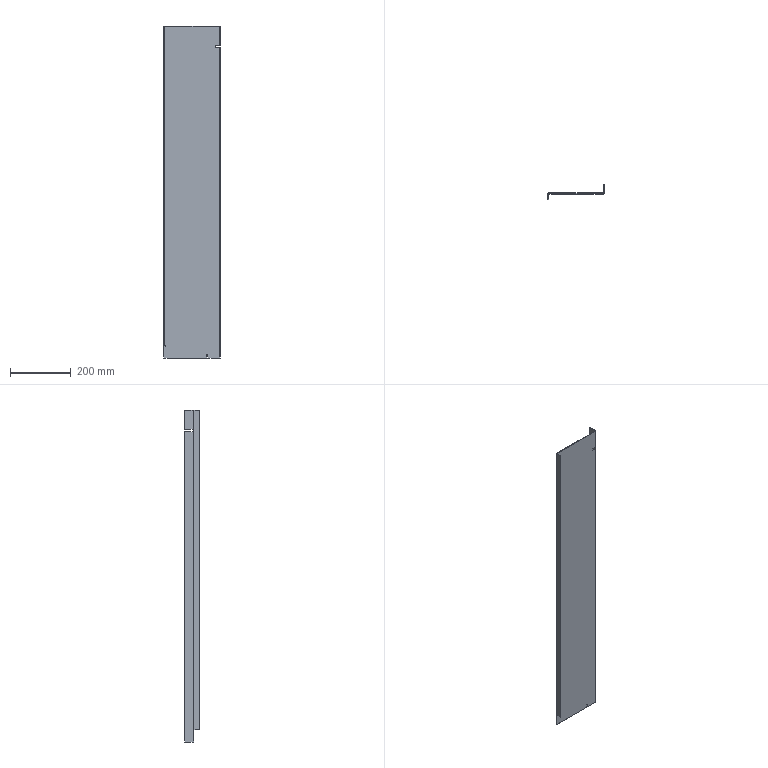Part | STEP file | Right Base Frame | 1 solid | 30 faces | box 185 x 48 x 1095 mm | volume 500987 mm3 | plane 23 | cylinder 7 | commonest cylinder face diameters 1 x4 5 x3
STEP:
#1=CARTESIAN_POINT('',(35.894,0.,57.218));
#2=VERTEX_POINT('',#1);
#3=CARTESIAN_POINT('',(35.894,0.,-966.782));
#4=VERTEX_POINT('',#3);
#5=CARTESIAN_POINT('',(35.894,0.,0.));
#6=DIRECTION('',(0.,0.,-1.));
#7=VECTOR('',#6,1000.);
#8=LINE('',#5,#7);
#9=EDGE_CURVE('',#2,#4,#8,.T.);
#10=ORIENTED_EDGE('',*,*,#9,.T.);
#11=CARTESIAN_POINT('',(-1.606,0.,-966.782));
#12=VERTEX_POINT('',#11);
#13=CARTESIAN_POINT('',(0.,0.,-966.782));
#14=DIRECTION('',(-1.,0.,0.));
#15=VECTOR('',#14,1000.);
#16=LINE('',#13,#15);
#17=EDGE_CURVE('',#4,#12,#16,.T.);
#18=ORIENTED_EDGE('',*,*,#17,.T.);
#19=CARTESIAN_POINT('',(-1.606,0.,-956.782));
#20=VERTEX_POINT('',#19);
#21=CARTESIAN_POINT('',(-1.606,0.,0.));
#22=DIRECTION('',(0.,0.,1.));
#23=VECTOR('',#22,1000.);
#24=LINE('',#21,#23);
#25=EDGE_CURVE('',#12,#20,#24,.T.);
#26=ORIENTED_EDGE('',*,*,#25,.T.);
#27=CARTESIAN_POINT('',(-5.606,0.,-956.782));
#28=VERTEX_POINT('',#27);
#29=CARTESIAN_POINT('',(0.,0.,-956.782));
#30=DIRECTION('',(-1.,0.,0.));
#31=VECTOR('',#30,1000.);
#32=LINE('',#29,#31);
#33=EDGE_CURVE('',#20,#28,#32,.T.);
#34=ORIENTED_EDGE('',*,*,#33,.T.);
#35=CARTESIAN_POINT('',(-5.606,0.,-966.782));
#36=VERTEX_POINT('',#35);
#37=CARTESIAN_POINT('',(-5.606,0.,0.));
#38=DIRECTION('',(0.,0.,-1.));
#39=VECTOR('',#38,1000.);
#40=LINE('',#37,#39);
#41=EDGE_CURVE('',#28,#36,#40,.T.);
#42=ORIENTED_EDGE('',*,*,#41,.T.);
#43=CARTESIAN_POINT('',(-146.606,0.,-966.782));
#44=VERTEX_POINT('',#43);
#45=CARTESIAN_POINT('',(0.,0.,-966.782));
#46=DIRECTION('',(-1.,0.,0.));
#47=VECTOR('',#46,1000.);
#48=LINE('',#45,#47);
#49=EDGE_CURVE('',#36,#44,#48,.T.);
#50=ORIENTED_EDGE('',*,*,#49,.T.);
#51=CARTESIAN_POINT('',(-146.606,0.,-927.782));
#52=VERTEX_POINT('',#51);
#53=CARTESIAN_POINT('',(-146.606,0.,0.));
#54=DIRECTION('',(0.,0.,1.));
#55=VECTOR('',#54,1000.);
#56=LINE('',#53,#55);
#57=EDGE_CURVE('',#44,#52,#56,.T.);
#58=ORIENTED_EDGE('',*,*,#57,.T.);
#59=CARTESIAN_POINT('',(-143.106,0.,-927.782));
#60=VERTEX_POINT('',#59);
#61=CARTESIAN_POINT('',(0.,0.,-927.782));
#62=DIRECTION('',(1.,0.,0.));
#63=VECTOR('',#62,1000.);
#64=LINE('',#61,#63);
#65=EDGE_CURVE('',#52,#60,#64,.T.);
#66=ORIENTED_EDGE('',*,*,#65,.T.);
#67=CARTESIAN_POINT('',(-143.106,0.,-926.782));
#68=VERTEX_POINT('',#67);
#69=CARTESIAN_POINT('',(-143.106,0.,-927.282));
#70=DIRECTION('',(0.,-1.,0.));
#71=DIRECTION('',(0.,0.,1.));
#72=AXIS2_PLACEMENT_3D('',#69,#70,#71);
#73=CIRCLE('',#72,0.5);
#74=EDGE_CURVE('',#60,#68,#73,.T.);
#75=ORIENTED_EDGE('',*,*,#74,.T.);
#76=CARTESIAN_POINT('',(-144.106,0.,-926.782));
#77=VERTEX_POINT('',#76);
#78=CARTESIAN_POINT('',(-143.106,0.,-926.782));
#79=DIRECTION('',(1.,0.,0.));
#80=VECTOR('',#79,1000.);
#81=LINE('',#78,#80);
#82=EDGE_CURVE('',#77,#68,#81,.T.);
#83=ORIENTED_EDGE('',*,*,#82,.F.);
#84=CARTESIAN_POINT('',(-144.106,0.,128.218));
#85=VERTEX_POINT('',#84);
#86=CARTESIAN_POINT('',(-144.106,0.,0.));
#87=DIRECTION('',(0.,0.,1.));
#88=VECTOR('',#87,1000.);
#89=LINE('',#86,#88);
#90=EDGE_CURVE('',#77,#85,#89,.T.);
#91=ORIENTED_EDGE('',*,*,#90,.T.);
#92=CARTESIAN_POINT('',(35.894,0.,128.218));
#93=VERTEX_POINT('',#92);
#94=CARTESIAN_POINT('',(0.,0.,128.218));
#95=DIRECTION('',(1.,0.,0.));
#96=VECTOR('',#95,1000.);
#97=LINE('',#94,#96);
#98=EDGE_CURVE('',#85,#93,#97,.T.);
#99=ORIENTED_EDGE('',*,*,#98,.T.);
#100=CARTESIAN_POINT('',(35.894,0.,64.218));
#101=VERTEX_POINT('',#100);
#102=CARTESIAN_POINT('',(35.894,0.,0.));
#103=DIRECTION('',(0.,0.,-1.));
#104=VECTOR('',#103,1000.);
#105=LINE('',#102,#104);
#106=EDGE_CURVE('',#93,#101,#105,.T.);
#107=ORIENTED_EDGE('',*,*,#106,.T.);
#108=CARTESIAN_POINT('',(22.394,0.,64.218));
#109=VERTEX_POINT('',#108);
#110=CARTESIAN_POINT('',(0.,0.,64.218));
#111=DIRECTION('',(-1.,0.,0.));
#112=VECTOR('',#111,1000.);
#113=LINE('',#110,#112);
#114=EDGE_CURVE('',#101,#109,#113,.T.);
#115=ORIENTED_EDGE('',*,*,#114,.T.);
#116=CARTESIAN_POINT('',(22.394,0.,57.218));
#117=VERTEX_POINT('',#116);
#118=CARTESIAN_POINT('',(22.394,0.,0.));
#119=DIRECTION('',(0.,0.,-1.));
#120=VECTOR('',#119,1000.);
#121=LINE('',#118,#120);
#122=EDGE_CURVE('',#109,#117,#121,.T.);
#123=ORIENTED_EDGE('',*,*,#122,.T.);
#124=CARTESIAN_POINT('',(0.,0.,57.218));
#125=DIRECTION('',(1.,0.,0.));
#126=VECTOR('',#125,1000.);
#127=LINE('',#124,#126);
#128=EDGE_CURVE('',#117,#2,#127,.T.);
#129=ORIENTED_EDGE('',*,*,#128,.T.);
#130=EDGE_LOOP('',(#10,#18,#26,#34,#42,#50,#58,#66,#75,#83,#91,#99,#107,#115,#123,#129));
#131=FACE_OUTER_BOUND('',#130,.T.);
#132=CARTESIAN_POINT('',(0.,0.,0.));
#133=DIRECTION('',(0.,1.,0.));
#134=DIRECTION('',(0.,0.,1.));
#135=AXIS2_PLACEMENT_3D('',#132,#133,#134);
#136=PLANE('',#135);
#137=ADVANCED_FACE('',(#131),#136,.T.);
#138=ORIENTED_EDGE('',*,*,#17,.F.);
#139=CARTESIAN_POINT('',(36.394,0.5,-966.782));
#140=VERTEX_POINT('',#139);
#141=CARTESIAN_POINT('',(35.894,0.5,-966.782));
#142=DIRECTION('',(0.,0.,1.));
#143=DIRECTION('',(-1.,0.,0.));
#144=AXIS2_PLACEMENT_3D('',#141,#142,#143);
#145=CIRCLE('',#144,0.5);
#146=EDGE_CURVE('',#4,#140,#145,.T.);
#147=ORIENTED_EDGE('',*,*,#146,.T.);
#148=CARTESIAN_POINT('',(36.394,28.,-966.782));
#149=VERTEX_POINT('',#148);
#150=CARTESIAN_POINT('',(36.394,0.,-966.782));
#151=DIRECTION('',(0.,-1.,0.));
#152=VECTOR('',#151,1000.);
#153=LINE('',#150,#152);
#154=EDGE_CURVE('',#149,#140,#153,.T.);
#155=ORIENTED_EDGE('',*,*,#154,.F.);
#156=CARTESIAN_POINT('',(38.394,28.,-966.782));
#157=VERTEX_POINT('',#156);
#158=CARTESIAN_POINT('',(38.394,28.,-966.782));
#159=DIRECTION('',(1.,0.,0.));
#160=VECTOR('',#159,1000.);
#161=LINE('',#158,#160);
#162=EDGE_CURVE('',#149,#157,#161,.T.);
#163=ORIENTED_EDGE('',*,*,#162,.T.);
#164=CARTESIAN_POINT('',(38.394,0.5,-966.782));
#165=VERTEX_POINT('',#164);
#166=CARTESIAN_POINT('',(38.394,0.,-966.782));
#167=DIRECTION('',(0.,-1.,0.));
#168=VECTOR('',#167,1000.);
#169=LINE('',#166,#168);
#170=EDGE_CURVE('',#157,#165,#169,.T.);
#171=ORIENTED_EDGE('',*,*,#170,.T.);
#172=CARTESIAN_POINT('',(35.894,-2.,-966.782));
#173=VERTEX_POINT('',#172);
#174=CARTESIAN_POINT('',(35.894,0.5,-966.782));
#175=DIRECTION('',(0.,0.,1.));
#176=DIRECTION('',(-1.,0.,0.));
#177=AXIS2_PLACEMENT_3D('',#174,#175,#176);
#178=CIRCLE('',#177,2.5);
#179=EDGE_CURVE('',#173,#165,#178,.T.);
#180=ORIENTED_EDGE('',*,*,#179,.F.);
#181=CARTESIAN_POINT('',(-1.606,-2.,-966.782));
#182=VERTEX_POINT('',#181);
#183=CARTESIAN_POINT('',(-146.606,-2.,-966.782));
#184=DIRECTION('',(-1.,0.,0.));
#185=VECTOR('',#184,1000.);
#186=LINE('',#183,#185);
#187=EDGE_CURVE('',#173,#182,#186,.T.);
#188=ORIENTED_EDGE('',*,*,#187,.T.);
#189=CARTESIAN_POINT('',(-1.606,-2.,-966.782));
#190=DIRECTION('',(0.,1.,0.));
#191=VECTOR('',#190,1000.);
#192=LINE('',#189,#191);
#193=EDGE_CURVE('',#182,#12,#192,.T.);
#194=ORIENTED_EDGE('',*,*,#193,.T.);
#195=EDGE_LOOP('',(#138,#147,#155,#163,#171,#180,#188,#194));
#196=FACE_OUTER_BOUND('',#195,.T.);
#197=CARTESIAN_POINT('',(-146.606,-2.,-966.782));
#198=DIRECTION('',(0.,0.,-1.));
#199=DIRECTION('',(-1.,0.,0.));
#200=AXIS2_PLACEMENT_3D('',#197,#198,#199);
#201=PLANE('',#200);
#202=ADVANCED_FACE('',(#196),#201,.T.);
#203=CARTESIAN_POINT('',(36.394,0.5,57.218));
#204=VERTEX_POINT('',#203);
#205=CARTESIAN_POINT('',(35.894,0.5,57.218));
#206=DIRECTION('',(0.,0.,-1.));
#207=DIRECTION('',(-1.,0.,0.));
#208=AXIS2_PLACEMENT_3D('',#205,#206,#207);
#209=CIRCLE('',#208,0.5);
#210=EDGE_CURVE('',#204,#2,#209,.T.);
#211=ORIENTED_EDGE('',*,*,#210,.F.);
#212=CARTESIAN_POINT('',(36.394,0.5,-966.782));
#213=DIRECTION('',(0.,0.,1.));
#214=VECTOR('',#213,1000.);
#215=LINE('',#212,#214);
#216=EDGE_CURVE('',#140,#204,#215,.T.);
#217=ORIENTED_EDGE('',*,*,#216,.F.);
#218=ORIENTED_EDGE('',*,*,#146,.F.);
#219=ORIENTED_EDGE('',*,*,#9,.F.);
#220=EDGE_LOOP('',(#211,#217,#218,#219));
#221=FACE_OUTER_BOUND('',#220,.T.);
#222=CARTESIAN_POINT('',(35.894,0.5,-966.782));
#223=DIRECTION('',(0.,0.,-1.));
#224=DIRECTION('',(-1.,0.,0.));
#225=AXIS2_PLACEMENT_3D('',#222,#223,#224);
#226=CYLINDRICAL_SURFACE('',#225,0.5);
#227=ADVANCED_FACE('',(#221),#226,.F.);
#228=CARTESIAN_POINT('',(38.394,28.,57.218));
#229=VERTEX_POINT('',#228);
#230=CARTESIAN_POINT('',(38.394,0.5,57.218));
#231=VERTEX_POINT('',#230);
#232=CARTESIAN_POINT('',(38.394,-20.,57.218));
#233=DIRECTION('',(0.,-1.,0.));
#234=VECTOR('',#233,1000.);
#235=LINE('',#232,#234);
#236=EDGE_CURVE('',#229,#231,#235,.T.);
#237=ORIENTED_EDGE('',*,*,#236,.F.);
#238=CARTESIAN_POINT('',(36.394,28.,57.218));
#239=VERTEX_POINT('',#238);
#240=CARTESIAN_POINT('',(38.394,28.,57.218));
#241=DIRECTION('',(1.,0.,0.));
#242=VECTOR('',#241,1000.);
#243=LINE('',#240,#242);
#244=EDGE_CURVE('',#239,#229,#243,.T.);
#245=ORIENTED_EDGE('',*,*,#244,.F.);
#246=CARTESIAN_POINT('',(36.394,-20.,57.218));
#247=DIRECTION('',(0.,1.,0.));
#248=VECTOR('',#247,1000.);
#249=LINE('',#246,#248);
#250=EDGE_CURVE('',#204,#239,#249,.T.);
#251=ORIENTED_EDGE('',*,*,#250,.F.);
#252=ORIENTED_EDGE('',*,*,#210,.T.);
#253=ORIENTED_EDGE('',*,*,#128,.F.);
#254=CARTESIAN_POINT('',(22.394,-2.,57.218));
#255=VERTEX_POINT('',#254);
#256=CARTESIAN_POINT('',(22.394,-20.,57.218));
#257=DIRECTION('',(0.,1.,0.));
#258=VECTOR('',#257,1000.);
#259=LINE('',#256,#258);
#260=EDGE_CURVE('',#255,#117,#259,.T.);
#261=ORIENTED_EDGE('',*,*,#260,.F.);
#262=CARTESIAN_POINT('',(35.894,-2.,57.218));
#263=VERTEX_POINT('',#262);
#264=CARTESIAN_POINT('',(38.394,-2.,57.218));
#265=DIRECTION('',(-1.,0.,0.));
#266=VECTOR('',#265,1000.);
#267=LINE('',#264,#266);
#268=EDGE_CURVE('',#263,#255,#267,.T.);
#269=ORIENTED_EDGE('',*,*,#268,.F.);
#270=CARTESIAN_POINT('',(35.894,0.5,57.218));
#271=DIRECTION('',(0.,0.,-1.));
#272=DIRECTION('',(-1.,0.,0.));
#273=AXIS2_PLACEMENT_3D('',#270,#271,#272);
#274=CIRCLE('',#273,2.5);
#275=EDGE_CURVE('',#231,#263,#274,.T.);
#276=ORIENTED_EDGE('',*,*,#275,.F.);
#277=EDGE_LOOP('',(#237,#245,#251,#252,#253,#261,#269,#276));
#278=FACE_OUTER_BOUND('',#277,.T.);
#279=CARTESIAN_POINT('',(38.394,-20.,57.218));
#280=DIRECTION('',(0.,0.,-1.));
#281=DIRECTION('',(-1.,0.,0.));
#282=AXIS2_PLACEMENT_3D('',#279,#280,#281);
#283=PLANE('',#282);
#284=ADVANCED_FACE('',(#278),#283,.F.);
#285=ORIENTED_EDGE('',*,*,#122,.F.);
#286=CARTESIAN_POINT('',(22.394,-2.,64.218));
#287=VERTEX_POINT('',#286);
#288=CARTESIAN_POINT('',(22.394,-20.,64.218));
#289=DIRECTION('',(0.,1.,0.));
#290=VECTOR('',#289,1000.);
#291=LINE('',#288,#290);
#292=EDGE_CURVE('',#287,#109,#291,.T.);
#293=ORIENTED_EDGE('',*,*,#292,.F.);
#294=CARTESIAN_POINT('',(22.394,-2.,57.218));
#295=DIRECTION('',(0.,0.,1.));
#296=VECTOR('',#295,1000.);
#297=LINE('',#294,#296);
#298=EDGE_CURVE('',#255,#287,#297,.T.);
#299=ORIENTED_EDGE('',*,*,#298,.F.);
#300=ORIENTED_EDGE('',*,*,#260,.T.);
#301=EDGE_LOOP('',(#285,#293,#299,#300));
#302=FACE_OUTER_BOUND('',#301,.T.);
#303=CARTESIAN_POINT('',(22.394,-20.,57.218));
#304=DIRECTION('',(-1.,0.,0.));
#305=DIRECTION('',(0.,-1.,0.));
#306=AXIS2_PLACEMENT_3D('',#303,#304,#305);
#307=PLANE('',#306);
#308=ADVANCED_FACE('',(#302),#307,.F.);
#309=ORIENTED_EDGE('',*,*,#114,.F.);
#310=CARTESIAN_POINT('',(36.394,0.5,64.218));
#311=VERTEX_POINT('',#310);
#312=CARTESIAN_POINT('',(35.894,0.5,64.218));
#313=DIRECTION('',(0.,0.,-1.));
#314=DIRECTION('',(-1.,0.,0.));
#315=AXIS2_PLACEMENT_3D('',#312,#313,#314);
#316=CIRCLE('',#315,0.5);
#317=EDGE_CURVE('',#311,#101,#316,.T.);
#318=ORIENTED_EDGE('',*,*,#317,.F.);
#319=CARTESIAN_POINT('',(36.394,28.,64.218));
#320=VERTEX_POINT('',#319);
#321=CARTESIAN_POINT('',(36.394,-20.,64.218));
#322=DIRECTION('',(0.,-1.,0.));
#323=VECTOR('',#322,1000.);
#324=LINE('',#321,#323);
#325=EDGE_CURVE('',#320,#311,#324,.T.);
#326=ORIENTED_EDGE('',*,*,#325,.F.);
#327=CARTESIAN_POINT('',(38.394,28.,64.218));
#328=VERTEX_POINT('',#327);
#329=CARTESIAN_POINT('',(38.394,28.,64.218));
#330=DIRECTION('',(-1.,0.,0.));
#331=VECTOR('',#330,1000.);
#332=LINE('',#329,#331);
#333=EDGE_CURVE('',#328,#320,#332,.T.);
#334=ORIENTED_EDGE('',*,*,#333,.F.);
#335=CARTESIAN_POINT('',(38.394,0.5,64.218));
#336=VERTEX_POINT('',#335);
#337=CARTESIAN_POINT('',(38.394,-20.,64.218));
#338=DIRECTION('',(0.,1.,0.));
#339=VECTOR('',#338,1000.);
#340=LINE('',#337,#339);
#341=EDGE_CURVE('',#336,#328,#340,.T.);
#342=ORIENTED_EDGE('',*,*,#341,.F.);
#343=CARTESIAN_POINT('',(35.894,-2.,64.218));
#344=VERTEX_POINT('',#343);
#345=CARTESIAN_POINT('',(35.894,0.5,64.218));
#346=DIRECTION('',(0.,0.,1.));
#347=DIRECTION('',(-1.,0.,0.));
#348=AXIS2_PLACEMENT_3D('',#345,#346,#347);
#349=CIRCLE('',#348,2.5);
#350=EDGE_CURVE('',#344,#336,#349,.T.);
#351=ORIENTED_EDGE('',*,*,#350,.F.);
#352=CARTESIAN_POINT('',(38.394,-2.,64.218));
#353=DIRECTION('',(1.,0.,0.));
#354=VECTOR('',#353,1000.);
#355=LINE('',#352,#354);
#356=EDGE_CURVE('',#287,#344,#355,.T.);
#357=ORIENTED_EDGE('',*,*,#356,.F.);
#358=ORIENTED_EDGE('',*,*,#292,.T.);
#359=EDGE_LOOP('',(#309,#318,#326,#334,#342,#351,#357,#358));
#360=FACE_OUTER_BOUND('',#359,.T.);
#361=CARTESIAN_POINT('',(38.394,-20.,64.218));
#362=DIRECTION('',(0.,0.,1.));
#363=DIRECTION('',(0.,-1.,0.));
#364=AXIS2_PLACEMENT_3D('',#361,#362,#363);
#365=PLANE('',#364);
#366=ADVANCED_FACE('',(#360),#365,.F.);
#367=ORIENTED_EDGE('',*,*,#317,.T.);
#368=ORIENTED_EDGE('',*,*,#106,.F.);
#369=CARTESIAN_POINT('',(36.394,0.5,128.218));
#370=VERTEX_POINT('',#369);
#371=CARTESIAN_POINT('',(35.894,0.5,128.218));
#372=DIRECTION('',(0.,0.,-1.));
#373=DIRECTION('',(-1.,0.,0.));
#374=AXIS2_PLACEMENT_3D('',#371,#372,#373);
#375=CIRCLE('',#374,0.5);
#376=EDGE_CURVE('',#370,#93,#375,.T.);
#377=ORIENTED_EDGE('',*,*,#376,.F.);
#378=CARTESIAN_POINT('',(36.394,0.5,-966.782));
#379=DIRECTION('',(0.,0.,1.));
#380=VECTOR('',#379,1000.);
#381=LINE('',#378,#380);
#382=EDGE_CURVE('',#311,#370,#381,.T.);
#383=ORIENTED_EDGE('',*,*,#382,.F.);
#384=EDGE_LOOP('',(#367,#368,#377,#383));
#385=FACE_OUTER_BOUND('',#384,.T.);
#386=CARTESIAN_POINT('',(35.894,0.5,-966.782));
#387=DIRECTION('',(0.,0.,-1.));
#388=DIRECTION('',(-1.,0.,0.));
#389=AXIS2_PLACEMENT_3D('',#386,#387,#388);
#390=CYLINDRICAL_SURFACE('',#389,0.5);
#391=ADVANCED_FACE('',(#385),#390,.F.);
#392=ORIENTED_EDGE('',*,*,#98,.F.);
#393=CARTESIAN_POINT('',(-146.606,-2.5,128.218));
#394=VERTEX_POINT('',#393);
#395=CARTESIAN_POINT('',(-144.106,-2.5,128.218));
#396=DIRECTION('',(0.,0.,-1.));
#397=DIRECTION('',(0.,1.,0.));
#398=AXIS2_PLACEMENT_3D('',#395,#396,#397);
#399=CIRCLE('',#398,2.5);
#400=EDGE_CURVE('',#394,#85,#399,.T.);
#401=ORIENTED_EDGE('',*,*,#400,.F.);
#402=CARTESIAN_POINT('',(-146.606,-20.,128.218));
#403=VERTEX_POINT('',#402);
#404=CARTESIAN_POINT('',(-146.606,0.,128.218));
#405=DIRECTION('',(0.,1.,0.));
#406=VECTOR('',#405,1000.);
#407=LINE('',#404,#406);
#408=EDGE_CURVE('',#403,#394,#407,.T.);
#409=ORIENTED_EDGE('',*,*,#408,.F.);
#410=CARTESIAN_POINT('',(-144.606,-20.,128.218));
#411=VERTEX_POINT('',#410);
#412=CARTESIAN_POINT('',(-146.606,-20.,128.218));
#413=DIRECTION('',(1.,0.,0.));
#414=VECTOR('',#413,1000.);
#415=LINE('',#412,#414);
#416=EDGE_CURVE('',#403,#411,#415,.T.);
#417=ORIENTED_EDGE('',*,*,#416,.T.);
#418=CARTESIAN_POINT('',(-144.606,-2.5,128.218));
#419=VERTEX_POINT('',#418);
#420=CARTESIAN_POINT('',(-144.606,-20.,128.218));
#421=DIRECTION('',(0.,1.,0.));
#422=VECTOR('',#421,1000.);
#423=LINE('',#420,#422);
#424=EDGE_CURVE('',#411,#419,#423,.T.);
#425=ORIENTED_EDGE('',*,*,#424,.T.);
#426=CARTESIAN_POINT('',(-144.106,-2.,128.218));
#427=VERTEX_POINT('',#426);
#428=CARTESIAN_POINT('',(-144.106,-2.5,128.218));
#429=DIRECTION('',(0.,0.,-1.));
#430=DIRECTION('',(0.,1.,0.));
#431=AXIS2_PLACEMENT_3D('',#428,#429,#430);
#432=CIRCLE('',#431,0.5);
#433=EDGE_CURVE('',#419,#427,#432,.T.);
#434=ORIENTED_EDGE('',*,*,#433,.T.);
#435=CARTESIAN_POINT('',(35.894,-2.,128.218));
#436=VERTEX_POINT('',#435);
#437=CARTESIAN_POINT('',(-146.606,-2.,128.218));
#438=DIRECTION('',(1.,0.,0.));
#439=VECTOR('',#438,1000.);
#440=LINE('',#437,#439);
#441=EDGE_CURVE('',#427,#436,#440,.T.);
#442=ORIENTED_EDGE('',*,*,#441,.T.);
#443=CARTESIAN_POINT('',(38.394,0.5,128.218));
#444=VERTEX_POINT('',#443);
#445=CARTESIAN_POINT('',(35.894,0.5,128.218));
#446=DIRECTION('',(0.,0.,-1.));
#447=DIRECTION('',(-1.,0.,0.));
#448=AXIS2_PLACEMENT_3D('',#445,#446,#447);
#449=CIRCLE('',#448,2.5);
#450=EDGE_CURVE('',#444,#436,#449,.T.);
#451=ORIENTED_EDGE('',*,*,#450,.F.);
#452=CARTESIAN_POINT('',(38.394,28.,128.218));
#453=VERTEX_POINT('',#452);
#454=CARTESIAN_POINT('',(38.394,0.,128.218));
#455=DIRECTION('',(0.,1.,0.));
#456=VECTOR('',#455,1000.);
#457=LINE('',#454,#456);
#458=EDGE_CURVE('',#444,#453,#457,.T.);
#459=ORIENTED_EDGE('',*,*,#458,.T.);
#460=CARTESIAN_POINT('',(36.394,28.,128.218));
#461=VERTEX_POINT('',#460);
#462=CARTESIAN_POINT('',(38.394,28.,128.218));
#463=DIRECTION('',(-1.,0.,0.));
#464=VECTOR('',#463,1000.);
#465=LINE('',#462,#464);
#466=EDGE_CURVE('',#453,#461,#465,.T.);
#467=ORIENTED_EDGE('',*,*,#466,.T.);
#468=CARTESIAN_POINT('',(36.394,0.,128.218));
#469=DIRECTION('',(0.,1.,0.));
#470=VECTOR('',#469,1000.);
#471=LINE('',#468,#470);
#472=EDGE_CURVE('',#370,#461,#471,.T.);
#473=ORIENTED_EDGE('',*,*,#472,.F.);
#474=ORIENTED_EDGE('',*,*,#376,.T.);
#475=EDGE_LOOP('',(#392,#401,#409,#417,#425,#434,#442,#451,#459,#467,#473,#474));
#476=FACE_OUTER_BOUND('',#475,.T.);
#477=CARTESIAN_POINT('',(-146.606,-2.,128.218));
#478=DIRECTION('',(0.,0.,1.));
#479=DIRECTION('',(1.,0.,0.));
#480=AXIS2_PLACEMENT_3D('',#477,#478,#479);
#481=PLANE('',#480);
#482=ADVANCED_FACE('',(#476),#481,.T.);
#483=CARTESIAN_POINT('',(-146.606,-2.5,-926.782));
#484=VERTEX_POINT('',#483);
#485=CARTESIAN_POINT('',(-146.606,-2.5,-926.782));
#486=DIRECTION('',(0.,0.,1.));
#487=VECTOR('',#486,1000.);
#488=LINE('',#485,#487);
#489=EDGE_CURVE('',#484,#394,#488,.T.);
#490=ORIENTED_EDGE('',*,*,#489,.T.);
#491=ORIENTED_EDGE('',*,*,#400,.T.);
#492=ORIENTED_EDGE('',*,*,#90,.F.);
#493=CARTESIAN_POINT('',(-144.106,-2.5,-926.782));
#494=DIRECTION('',(0.,0.,1.));
#495=DIRECTION('',(0.,1.,0.));
#496=AXIS2_PLACEMENT_3D('',#493,#494,#495);
#497=CIRCLE('',#496,2.5);
#498=EDGE_CURVE('',#77,#484,#497,.T.);
#499=ORIENTED_EDGE('',*,*,#498,.T.);
#500=EDGE_LOOP('',(#490,#491,#492,#499));
#501=FACE_OUTER_BOUND('',#500,.T.);
#502=CARTESIAN_POINT('',(-144.106,-2.5,-926.782));
#503=DIRECTION('',(0.,0.,-1.));
#504=DIRECTION('',(0.,1.,0.));
#505=AXIS2_PLACEMENT_3D('',#502,#503,#504);
#506=CYLINDRICAL_SURFACE('',#505,2.5);
#507=ADVANCED_FACE('',(#501),#506,.T.);
#508=CARTESIAN_POINT('',(-146.606,-2.,-927.782));
#509=VERTEX_POINT('',#508);
#510=CARTESIAN_POINT('',(-143.106,-2.,-927.782));
#511=VERTEX_POINT('',#510);
#512=CARTESIAN_POINT('',(-146.606,-2.,-927.782));
#513=DIRECTION('',(1.,0.,0.));
#514=VECTOR('',#513,1000.);
#515=LINE('',#512,#514);
#516=EDGE_CURVE('',#509,#511,#515,.T.);
#517=ORIENTED_EDGE('',*,*,#516,.T.);
#518=CARTESIAN_POINT('',(-143.106,-2.,-927.782));
#519=DIRECTION('',(0.,1.,0.));
#520=VECTOR('',#519,1000.);
#521=LINE('',#518,#520);
#522=EDGE_CURVE('',#511,#60,#521,.T.);
#523=ORIENTED_EDGE('',*,*,#522,.T.);
#524=ORIENTED_EDGE('',*,*,#65,.F.);
#525=CARTESIAN_POINT('',(-146.606,-2.,-927.782));
#526=DIRECTION('',(0.,-1.,0.));
#527=VECTOR('',#526,1000.);
#528=LINE('',#525,#527);
#529=EDGE_CURVE('',#52,#509,#528,.T.);
#530=ORIENTED_EDGE('',*,*,#529,.T.);
#531=EDGE_LOOP('',(#517,#523,#524,#530));
#532=FACE_OUTER_BOUND('',#531,.T.);
#533=CARTESIAN_POINT('',(-146.606,-2.,-927.782));
#534=DIRECTION('',(0.,0.,1.));
#535=DIRECTION('',(0.,-1.,0.));
#536=AXIS2_PLACEMENT_3D('',#533,#534,#535);
#537=PLANE('',#536);
#538=ADVANCED_FACE('',(#532),#537,.T.);
#539=ORIENTED_EDGE('',*,*,#57,.F.);
#540=CARTESIAN_POINT('',(-146.606,-2.,-966.782));
#541=VERTEX_POINT('',#540);
#542=CARTESIAN_POINT('',(-146.606,-2.,-966.782));
#543=DIRECTION('',(0.,-1.,0.));
#544=VECTOR('',#543,1000.);
#545=LINE('',#542,#544);
#546=EDGE_CURVE('',#44,#541,#545,.T.);
#547=ORIENTED_EDGE('',*,*,#546,.T.);
#548=CARTESIAN_POINT('',(-146.606,-2.,-966.782));
#549=DIRECTION('',(0.,0.,1.));
#550=VECTOR('',#549,1000.);
#551=LINE('',#548,#550);
#552=EDGE_CURVE('',#541,#509,#551,.T.);
#553=ORIENTED_EDGE('',*,*,#552,.T.);
#554=ORIENTED_EDGE('',*,*,#529,.F.);
#555=EDGE_LOOP('',(#539,#547,#553,#554));
#556=FACE_OUTER_BOUND('',#555,.T.);
#557=CARTESIAN_POINT('',(-146.606,-2.,-966.782));
#558=DIRECTION('',(-1.,0.,0.));
#559=DIRECTION('',(0.,0.,1.));
#560=AXIS2_PLACEMENT_3D('',#557,#558,#559);
#561=PLANE('',#560);
#562=ADVANCED_FACE('',(#556),#561,.T.);
#563=ORIENTED_EDGE('',*,*,#546,.F.);
#564=ORIENTED_EDGE('',*,*,#49,.F.);
#565=CARTESIAN_POINT('',(-5.606,-2.,-966.782));
#566=VERTEX_POINT('',#565);
#567=CARTESIAN_POINT('',(-5.606,-2.,-966.782));
#568=DIRECTION('',(0.,-1.,0.));
#569=VECTOR('',#568,1000.);
#570=LINE('',#567,#569);
#571=EDGE_CURVE('',#36,#566,#570,.T.);
#572=ORIENTED_EDGE('',*,*,#571,.T.);
#573=CARTESIAN_POINT('',(-146.606,-2.,-966.782));
#574=DIRECTION('',(-1.,0.,0.));
#575=VECTOR('',#574,1000.);
#576=LINE('',#573,#575);
#577=EDGE_CURVE('',#566,#541,#576,.T.);
#578=ORIENTED_EDGE('',*,*,#577,.T.);
#579=EDGE_LOOP('',(#563,#564,#572,#578));
#580=FACE_OUTER_BOUND('',#579,.T.);
#581=CARTESIAN_POINT('',(-146.606,-2.,-966.782));
#582=DIRECTION('',(0.,0.,-1.));
#583=DIRECTION('',(-1.,0.,0.));
#584=AXIS2_PLACEMENT_3D('',#581,#582,#583);
#585=PLANE('',#584);
#586=ADVANCED_FACE('',(#580),#585,.T.);
#587=ORIENTED_EDGE('',*,*,#41,.F.);
#588=CARTESIAN_POINT('',(-5.606,-2.,-956.782));
#589=VERTEX_POINT('',#588);
#590=CARTESIAN_POINT('',(-5.606,-10.,-956.782));
#591=DIRECTION('',(0.,1.,0.));
#592=VECTOR('',#591,1000.);
#593=LINE('',#590,#592);
#594=EDGE_CURVE('',#589,#28,#593,.T.);
#595=ORIENTED_EDGE('',*,*,#594,.F.);
#596=CARTESIAN_POINT('',(-5.606,-2.,-966.782));
#597=DIRECTION('',(0.,0.,1.));
#598=VECTOR('',#597,1000.);
#599=LINE('',#596,#598);
#600=EDGE_CURVE('',#566,#589,#599,.T.);
#601=ORIENTED_EDGE('',*,*,#600,.F.);
#602=ORIENTED_EDGE('',*,*,#571,.F.);
#603=EDGE_LOOP('',(#587,#595,#601,#602));
#604=FACE_OUTER_BOUND('',#603,.T.);
#605=CARTESIAN_POINT('',(-5.606,-10.,-966.782));
#606=DIRECTION('',(-1.,0.,0.));
#607=DIRECTION('',(0.,0.,1.));
#608=AXIS2_PLACEMENT_3D('',#605,#606,#607);
#609=PLANE('',#608);
#610=ADVANCED_FACE('',(#604),#609,.F.);
#611=ORIENTED_EDGE('',*,*,#33,.F.);
#612=CARTESIAN_POINT('',(-1.606,-2.,-956.782));
#613=VERTEX_POINT('',#612);
#614=CARTESIAN_POINT('',(-1.606,-10.,-956.782));
#615=DIRECTION('',(0.,1.,0.));
#616=VECTOR('',#615,1000.);
#617=LINE('',#614,#616);
#618=EDGE_CURVE('',#613,#20,#617,.T.);
#619=ORIENTED_EDGE('',*,*,#618,.F.);
#620=CARTESIAN_POINT('',(-1.606,-2.,-956.782));
#621=DIRECTION('',(1.,0.,0.));
#622=VECTOR('',#621,1000.);
#623=LINE('',#620,#622);
#624=EDGE_CURVE('',#589,#613,#623,.T.);
#625=ORIENTED_EDGE('',*,*,#624,.F.);
#626=ORIENTED_EDGE('',*,*,#594,.T.);
#627=EDGE_LOOP('',(#611,#619,#625,#626));
#628=FACE_OUTER_BOUND('',#627,.T.);
#629=CARTESIAN_POINT('',(-1.606,-10.,-956.782));
#630=DIRECTION('',(0.,0.,1.));
#631=DIRECTION('',(1.,0.,0.));
#632=AXIS2_PLACEMENT_3D('',#629,#630,#631);
#633=PLANE('',#632);
#634=ADVANCED_FACE('',(#628),#633,.F.);
#635=ORIENTED_EDGE('',*,*,#25,.F.);
#636=ORIENTED_EDGE('',*,*,#193,.F.);
#637=CARTESIAN_POINT('',(-1.606,-2.,-966.782));
#638=DIRECTION('',(0.,0.,-1.));
#639=VECTOR('',#638,1000.);
#640=LINE('',#637,#639);
#641=EDGE_CURVE('',#613,#182,#640,.T.);
#642=ORIENTED_EDGE('',*,*,#641,.F.);
#643=ORIENTED_EDGE('',*,*,#618,.T.);
#644=EDGE_LOOP('',(#635,#636,#642,#643));
#645=FACE_OUTER_BOUND('',#644,.T.);
#646=CARTESIAN_POINT('',(-1.606,-10.,-966.782));
#647=DIRECTION('',(1.,0.,0.));
#648=DIRECTION('',(0.,0.,-1.));
#649=AXIS2_PLACEMENT_3D('',#646,#647,#648);
#650=PLANE('',#649);
#651=ADVANCED_FACE('',(#645),#650,.F.);
#652=ORIENTED_EDGE('',*,*,#641,.T.);
#653=ORIENTED_EDGE('',*,*,#187,.F.);
#654=CARTESIAN_POINT('',(35.894,-2.,0.));
#655=DIRECTION('',(0.,0.,-1.));
#656=VECTOR('',#655,1000.);
#657=LINE('',#654,#656);
#658=EDGE_CURVE('',#263,#173,#657,.T.);
#659=ORIENTED_EDGE('',*,*,#658,.F.);
#660=ORIENTED_EDGE('',*,*,#268,.T.);
#661=ORIENTED_EDGE('',*,*,#298,.T.);
#662=ORIENTED_EDGE('',*,*,#356,.T.);
#663=CARTESIAN_POINT('',(35.894,-2.,0.));
#664=DIRECTION('',(0.,0.,-1.));
#665=VECTOR('',#664,1000.);
#666=LINE('',#663,#665);
#667=EDGE_CURVE('',#436,#344,#666,.T.);
#668=ORIENTED_EDGE('',*,*,#667,.F.);
#669=ORIENTED_EDGE('',*,*,#441,.F.);
#670=CARTESIAN_POINT('',(-144.106,-2.,-926.782));
#671=VERTEX_POINT('',#670);
#672=CARTESIAN_POINT('',(-144.106,-2.,0.));
#673=DIRECTION('',(0.,0.,1.));
#674=VECTOR('',#673,1000.);
#675=LINE('',#672,#674);
#676=EDGE_CURVE('',#671,#427,#675,.T.);
#677=ORIENTED_EDGE('',*,*,#676,.F.);
#678=CARTESIAN_POINT('',(-143.106,-2.,-926.782));
#679=VERTEX_POINT('',#678);
#680=CARTESIAN_POINT('',(-143.106,-2.,-926.782));
#681=DIRECTION('',(-1.,0.,0.));
#682=VECTOR('',#681,1000.);
#683=LINE('',#680,#682);
#684=EDGE_CURVE('',#679,#671,#683,.T.);
#685=ORIENTED_EDGE('',*,*,#684,.F.);
#686=CARTESIAN_POINT('',(-143.106,-2.,-927.282));
#687=DIRECTION('',(0.,-1.,0.));
#688=DIRECTION('',(0.,0.,1.));
#689=AXIS2_PLACEMENT_3D('',#686,#687,#688);
#690=CIRCLE('',#689,0.5);
#691=EDGE_CURVE('',#511,#679,#690,.T.);
#692=ORIENTED_EDGE('',*,*,#691,.F.);
#693=ORIENTED_EDGE('',*,*,#516,.F.);
#694=ORIENTED_EDGE('',*,*,#552,.F.);
#695=ORIENTED_EDGE('',*,*,#577,.F.);
#696=ORIENTED_EDGE('',*,*,#600,.T.);
#697=ORIENTED_EDGE('',*,*,#624,.T.);
#698=EDGE_LOOP('',(#652,#653,#659,#660,#661,#662,#668,#669,#677,#685,#692,#693,#694,#695,#696,#697));
#699=FACE_OUTER_BOUND('',#698,.T.);
#700=CARTESIAN_POINT('',(0.,-2.,0.));
#701=DIRECTION('',(0.,1.,0.));
#702=DIRECTION('',(0.,0.,1.));
#703=AXIS2_PLACEMENT_3D('',#700,#701,#702);
#704=PLANE('',#703);
#705=ADVANCED_FACE('',(#699),#704,.F.);
#706=ORIENTED_EDGE('',*,*,#154,.T.);
#707=ORIENTED_EDGE('',*,*,#216,.T.);
#708=ORIENTED_EDGE('',*,*,#250,.T.);
#709=CARTESIAN_POINT('',(36.394,28.,0.));
#710=DIRECTION('',(0.,0.,-1.));
#711=VECTOR('',#710,1000.);
#712=LINE('',#709,#711);
#713=EDGE_CURVE('',#239,#149,#712,.T.);
#714=ORIENTED_EDGE('',*,*,#713,.T.);
#715=EDGE_LOOP('',(#706,#707,#708,#714));
#716=FACE_OUTER_BOUND('',#715,.T.);
#717=CARTESIAN_POINT('',(36.394,0.,0.));
#718=DIRECTION('',(-1.,0.,0.));
#719=DIRECTION('',(0.,-1.,0.));
#720=AXIS2_PLACEMENT_3D('',#717,#718,#719);
#721=PLANE('',#720);
#722=ADVANCED_FACE('',(#716),#721,.T.);
#723=ORIENTED_EDGE('',*,*,#179,.T.);
#724=CARTESIAN_POINT('',(38.394,0.5,-966.782));
#725=DIRECTION('',(0.,0.,1.));
#726=VECTOR('',#725,1000.);
#727=LINE('',#724,#726);
#728=EDGE_CURVE('',#165,#231,#727,.T.);
#729=ORIENTED_EDGE('',*,*,#728,.T.);
#730=ORIENTED_EDGE('',*,*,#275,.T.);
#731=ORIENTED_EDGE('',*,*,#658,.T.);
#732=EDGE_LOOP('',(#723,#729,#730,#731));
#733=FACE_OUTER_BOUND('',#732,.T.);
#734=CARTESIAN_POINT('',(35.894,0.5,-966.782));
#735=DIRECTION('',(0.,0.,-1.));
#736=DIRECTION('',(-1.,0.,0.));
#737=AXIS2_PLACEMENT_3D('',#734,#735,#736);
#738=CYLINDRICAL_SURFACE('',#737,2.5);
#739=ADVANCED_FACE('',(#733),#738,.T.);
#740=ORIENTED_EDGE('',*,*,#236,.T.);
#741=ORIENTED_EDGE('',*,*,#728,.F.);
#742=ORIENTED_EDGE('',*,*,#170,.F.);
#743=CARTESIAN_POINT('',(38.394,28.,0.));
#744=DIRECTION('',(0.,0.,-1.));
#745=VECTOR('',#744,1000.);
#746=LINE('',#743,#745);
#747=EDGE_CURVE('',#229,#157,#746,.T.);
#748=ORIENTED_EDGE('',*,*,#747,.F.);
#749=EDGE_LOOP('',(#740,#741,#742,#748));
#750=FACE_OUTER_BOUND('',#749,.T.);
#751=CARTESIAN_POINT('',(38.394,0.,0.));
#752=DIRECTION('',(-1.,0.,0.));
#753=DIRECTION('',(0.,-1.,0.));
#754=AXIS2_PLACEMENT_3D('',#751,#752,#753);
#755=PLANE('',#754);
#756=ADVANCED_FACE('',(#750),#755,.F.);
#757=ORIENTED_EDGE('',*,*,#244,.T.);
#758=ORIENTED_EDGE('',*,*,#747,.T.);
#759=ORIENTED_EDGE('',*,*,#162,.F.);
#760=ORIENTED_EDGE('',*,*,#713,.F.);
#761=EDGE_LOOP('',(#757,#758,#759,#760));
#762=FACE_OUTER_BOUND('',#761,.T.);
#763=CARTESIAN_POINT('',(38.394,28.,128.218));
#764=DIRECTION('',(0.,-1.,0.));
#765=DIRECTION('',(1.,0.,0.));
#766=AXIS2_PLACEMENT_3D('',#763,#764,#765);
#767=PLANE('',#766);
#768=ADVANCED_FACE('',(#762),#767,.F.);
#769=ORIENTED_EDGE('',*,*,#472,.T.);
#770=CARTESIAN_POINT('',(36.394,28.,0.));
#771=DIRECTION('',(0.,0.,-1.));
#772=VECTOR('',#771,1000.);
#773=LINE('',#770,#772);
#774=EDGE_CURVE('',#461,#320,#773,.T.);
#775=ORIENTED_EDGE('',*,*,#774,.T.);
#776=ORIENTED_EDGE('',*,*,#325,.T.);
#777=ORIENTED_EDGE('',*,*,#382,.T.);
#778=EDGE_LOOP('',(#769,#775,#776,#777));
#779=FACE_OUTER_BOUND('',#778,.T.);
#780=CARTESIAN_POINT('',(36.394,0.,0.));
#781=DIRECTION('',(-1.,0.,0.));
#782=DIRECTION('',(0.,-1.,0.));
#783=AXIS2_PLACEMENT_3D('',#780,#781,#782);
#784=PLANE('',#783);
#785=ADVANCED_FACE('',(#779),#784,.T.);
#786=ORIENTED_EDGE('',*,*,#333,.T.);
#787=ORIENTED_EDGE('',*,*,#774,.F.);
#788=ORIENTED_EDGE('',*,*,#466,.F.);
#789=CARTESIAN_POINT('',(38.394,28.,128.218));
#790=DIRECTION('',(0.,0.,1.));
#791=VECTOR('',#790,1000.);
#792=LINE('',#789,#791);
#793=EDGE_CURVE('',#328,#453,#792,.T.);
#794=ORIENTED_EDGE('',*,*,#793,.F.);
#795=EDGE_LOOP('',(#786,#787,#788,#794));
#796=FACE_OUTER_BOUND('',#795,.T.);
#797=CARTESIAN_POINT('',(38.394,28.,128.218));
#798=DIRECTION('',(0.,-1.,0.));
#799=DIRECTION('',(1.,0.,0.));
#800=AXIS2_PLACEMENT_3D('',#797,#798,#799);
#801=PLANE('',#800);
#802=ADVANCED_FACE('',(#796),#801,.F.);
#803=ORIENTED_EDGE('',*,*,#341,.T.);
#804=ORIENTED_EDGE('',*,*,#793,.T.);
#805=ORIENTED_EDGE('',*,*,#458,.F.);
#806=CARTESIAN_POINT('',(38.394,0.5,0.));
#807=DIRECTION('',(0.,0.,1.));
#808=VECTOR('',#807,1000.);
#809=LINE('',#806,#808);
#810=EDGE_CURVE('',#336,#444,#809,.T.);
#811=ORIENTED_EDGE('',*,*,#810,.F.);
#812=EDGE_LOOP('',(#803,#804,#805,#811));
#813=FACE_OUTER_BOUND('',#812,.T.);
#814=CARTESIAN_POINT('',(38.394,0.,0.));
#815=DIRECTION('',(-1.,0.,0.));
#816=DIRECTION('',(0.,-1.,0.));
#817=AXIS2_PLACEMENT_3D('',#814,#815,#816);
#818=PLANE('',#817);
#819=ADVANCED_FACE('',(#813),#818,.F.);
#820=ORIENTED_EDGE('',*,*,#450,.T.);
#821=ORIENTED_EDGE('',*,*,#667,.T.);
#822=ORIENTED_EDGE('',*,*,#350,.T.);
#823=ORIENTED_EDGE('',*,*,#810,.T.);
#824=EDGE_LOOP('',(#820,#821,#822,#823));
#825=FACE_OUTER_BOUND('',#824,.T.);
#826=CARTESIAN_POINT('',(35.894,0.5,-966.782));
#827=DIRECTION('',(0.,0.,-1.));
#828=DIRECTION('',(-1.,0.,0.));
#829=AXIS2_PLACEMENT_3D('',#826,#827,#828);
#830=CYLINDRICAL_SURFACE('',#829,2.5);
#831=ADVANCED_FACE('',(#825),#830,.T.);
#832=CARTESIAN_POINT('',(-146.606,-20.,-926.782));
#833=VERTEX_POINT('',#832);
#834=CARTESIAN_POINT('',(-146.606,0.,-926.782));
#835=DIRECTION('',(0.,-1.,0.));
#836=VECTOR('',#835,1000.);
#837=LINE('',#834,#836);
#838=EDGE_CURVE('',#484,#833,#837,.T.);
#839=ORIENTED_EDGE('',*,*,#838,.T.);
#840=CARTESIAN_POINT('',(-146.606,-20.,0.));
#841=DIRECTION('',(0.,0.,1.));
#842=VECTOR('',#841,1000.);
#843=LINE('',#840,#842);
#844=EDGE_CURVE('',#833,#403,#843,.T.);
#845=ORIENTED_EDGE('',*,*,#844,.T.);
#846=ORIENTED_EDGE('',*,*,#408,.T.);
#847=ORIENTED_EDGE('',*,*,#489,.F.);
#848=EDGE_LOOP('',(#839,#845,#846,#847));
#849=FACE_OUTER_BOUND('',#848,.T.);
#850=CARTESIAN_POINT('',(-146.606,0.,0.));
#851=DIRECTION('',(-1.,0.,0.));
#852=DIRECTION('',(0.,-1.,0.));
#853=AXIS2_PLACEMENT_3D('',#850,#851,#852);
#854=PLANE('',#853);
#855=ADVANCED_FACE('',(#849),#854,.T.);
#856=CARTESIAN_POINT('',(-144.606,-2.5,-926.782));
#857=VERTEX_POINT('',#856);
#858=CARTESIAN_POINT('',(-144.106,-2.5,-926.782));
#859=DIRECTION('',(0.,0.,-1.));
#860=DIRECTION('',(0.,1.,0.));
#861=AXIS2_PLACEMENT_3D('',#858,#859,#860);
#862=CIRCLE('',#861,0.5);
#863=EDGE_CURVE('',#857,#671,#862,.T.);
#864=ORIENTED_EDGE('',*,*,#863,.F.);
#865=CARTESIAN_POINT('',(-144.606,-20.,-926.782));
#866=VERTEX_POINT('',#865);
#867=CARTESIAN_POINT('',(-144.606,-2.,-926.782));
#868=DIRECTION('',(0.,-1.,0.));
#869=VECTOR('',#868,1000.);
#870=LINE('',#867,#869);
#871=EDGE_CURVE('',#857,#866,#870,.T.);
#872=ORIENTED_EDGE('',*,*,#871,.T.);
#873=CARTESIAN_POINT('',(-146.606,-20.,-926.782));
#874=DIRECTION('',(1.,0.,0.));
#875=VECTOR('',#874,1000.);
#876=LINE('',#873,#875);
#877=EDGE_CURVE('',#833,#866,#876,.T.);
#878=ORIENTED_EDGE('',*,*,#877,.F.);
#879=ORIENTED_EDGE('',*,*,#838,.F.);
#880=ORIENTED_EDGE('',*,*,#498,.F.);
#881=ORIENTED_EDGE('',*,*,#82,.T.);
#882=CARTESIAN_POINT('',(-143.106,-2.,-926.782));
#883=DIRECTION('',(0.,-1.,0.));
#884=VECTOR('',#883,1000.);
#885=LINE('',#882,#884);
#886=EDGE_CURVE('',#68,#679,#885,.T.);
#887=ORIENTED_EDGE('',*,*,#886,.T.);
#888=ORIENTED_EDGE('',*,*,#684,.T.);
#889=EDGE_LOOP('',(#864,#872,#878,#879,#880,#881,#887,#888));
#890=FACE_OUTER_BOUND('',#889,.T.);
#891=CARTESIAN_POINT('',(-144.106,-2.5,-926.782));
#892=DIRECTION('',(0.,0.,1.));
#893=DIRECTION('',(0.,-1.,0.));
#894=AXIS2_PLACEMENT_3D('',#891,#892,#893);
#895=PLANE('',#894);
#896=ADVANCED_FACE('',(#890),#895,.F.);
#897=ORIENTED_EDGE('',*,*,#522,.F.);
#898=ORIENTED_EDGE('',*,*,#691,.T.);
#899=ORIENTED_EDGE('',*,*,#886,.F.);
#900=ORIENTED_EDGE('',*,*,#74,.F.);
#901=EDGE_LOOP('',(#897,#898,#899,#900));
#902=FACE_OUTER_BOUND('',#901,.T.);
#903=CARTESIAN_POINT('',(-143.106,-2.,-927.282));
#904=DIRECTION('',(0.,1.,0.));
#905=DIRECTION('',(0.,0.,1.));
#906=AXIS2_PLACEMENT_3D('',#903,#904,#905);
#907=CYLINDRICAL_SURFACE('',#906,0.5);
#908=ADVANCED_FACE('',(#902),#907,.F.);
#909=ORIENTED_EDGE('',*,*,#433,.F.);
#910=CARTESIAN_POINT('',(-144.606,-2.5,-926.782));
#911=DIRECTION('',(0.,0.,1.));
#912=VECTOR('',#911,1000.);
#913=LINE('',#910,#912);
#914=EDGE_CURVE('',#857,#419,#913,.T.);
#915=ORIENTED_EDGE('',*,*,#914,.F.);
#916=ORIENTED_EDGE('',*,*,#863,.T.);
#917=ORIENTED_EDGE('',*,*,#676,.T.);
#918=EDGE_LOOP('',(#909,#915,#916,#917));
#919=FACE_OUTER_BOUND('',#918,.T.);
#920=CARTESIAN_POINT('',(-144.106,-2.5,-926.782));
#921=DIRECTION('',(0.,0.,-1.));
#922=DIRECTION('',(0.,1.,0.));
#923=AXIS2_PLACEMENT_3D('',#920,#921,#922);
#924=CYLINDRICAL_SURFACE('',#923,0.5);
#925=ADVANCED_FACE('',(#919),#924,.F.);
#926=ORIENTED_EDGE('',*,*,#844,.F.);
#927=ORIENTED_EDGE('',*,*,#877,.T.);
#928=CARTESIAN_POINT('',(-144.606,-20.,-926.782));
#929=DIRECTION('',(0.,0.,1.));
#930=VECTOR('',#929,1000.);
#931=LINE('',#928,#930);
#932=EDGE_CURVE('',#866,#411,#931,.T.);
#933=ORIENTED_EDGE('',*,*,#932,.T.);
#934=ORIENTED_EDGE('',*,*,#416,.F.);
#935=EDGE_LOOP('',(#926,#927,#933,#934));
#936=FACE_OUTER_BOUND('',#935,.T.);
#937=CARTESIAN_POINT('',(-146.606,-20.,-926.782));
#938=DIRECTION('',(0.,-1.,0.));
#939=DIRECTION('',(1.,0.,0.));
#940=AXIS2_PLACEMENT_3D('',#937,#938,#939);
#941=PLANE('',#940);
#942=ADVANCED_FACE('',(#936),#941,.T.);
#943=ORIENTED_EDGE('',*,*,#424,.F.);
#944=ORIENTED_EDGE('',*,*,#932,.F.);
#945=ORIENTED_EDGE('',*,*,#871,.F.);
#946=ORIENTED_EDGE('',*,*,#914,.T.);
#947=EDGE_LOOP('',(#943,#944,#945,#946));
#948=FACE_OUTER_BOUND('',#947,.T.);
#949=CARTESIAN_POINT('',(-144.606,0.,0.));
#950=DIRECTION('',(-1.,0.,0.));
#951=DIRECTION('',(0.,-1.,0.));
#952=AXIS2_PLACEMENT_3D('',#949,#950,#951);
#953=PLANE('',#952);
#954=ADVANCED_FACE('',(#948),#953,.F.);
#955=CLOSED_SHELL('',(#137,#202,#227,#284,#308,#366,#391,#482,#507,#538,#562,#586,#610,#634,#651,#705,#722,#739,#756,#768,#785,#802,#819,#831,#855,#896,#908,#925,#942,#954));
#956=MANIFOLD_SOLID_BREP('',#955);
#957=CARTESIAN_POINT('',(0.,0.,0.));
#958=DIRECTION('',(0.,0.,1.));
#959=DIRECTION('',(1.,0.,0.));
#960=AXIS2_PLACEMENT_3D('',#957,#958,#959);
#961=(LENGTH_UNIT()NAMED_UNIT(*)SI_UNIT(.MILLI.,.METRE.));
#962=UNCERTAINTY_MEASURE_WITH_UNIT(LENGTH_MEASURE(0.00001),#961,'','');
#963=(NAMED_UNIT(*)PLANE_ANGLE_UNIT()SI_UNIT($,.RADIAN.));
#964=(NAMED_UNIT(*)SI_UNIT($,.STERADIAN.)SOLID_ANGLE_UNIT());
#965=(GEOMETRIC_REPRESENTATION_CONTEXT(3)GLOBAL_UNCERTAINTY_ASSIGNED_CONTEXT((#962))GLOBAL_UNIT_ASSIGNED_CONTEXT((#961,#963,#964))REPRESENTATION_CONTEXT('',''));
#966=ADVANCED_BREP_SHAPE_REPRESENTATION('',(#956,#960),#965);